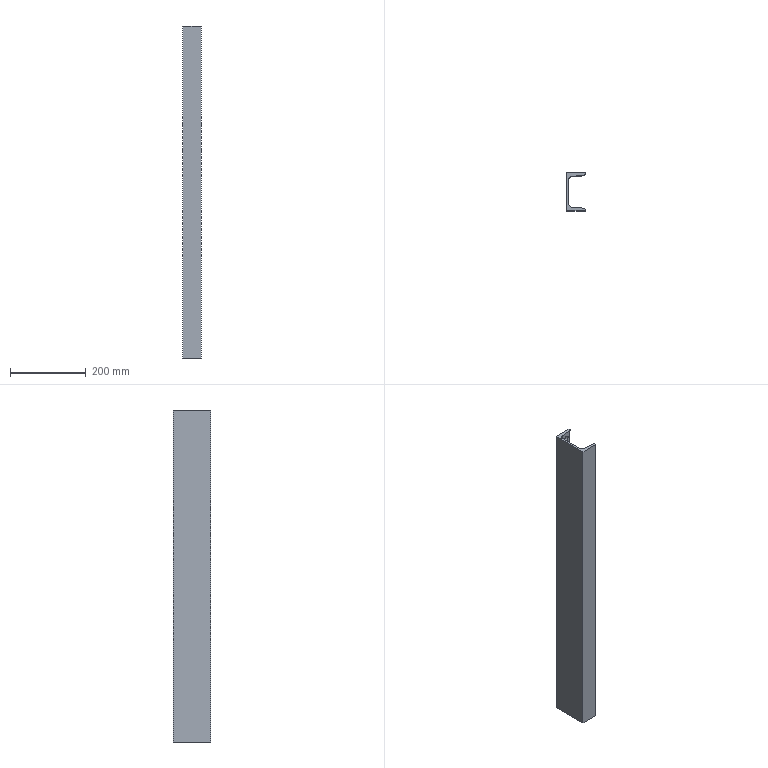Part | NX | features BREP 1, DATUM_CSYS 1, SKETCH 1 | 1 solid | 24 faces | box 48 x 100 x 876 mm | volume 1087998 mm3 | cylinder 14 | plane 10 | commonest cylinder face diameters 14 x10 8.4 x2 17 x2
STEP:
#1=CARTESIAN_POINT('',(30.,92.079,203.));
#2=VERTEX_POINT('',#1);
#3=CARTESIAN_POINT('',(30.,92.079,217.));
#4=VERTEX_POINT('',#3);
#5=CARTESIAN_POINT('',(30.,92.079,203.));
#6=CARTESIAN_POINT('',(16.,90.926,203.));
#7=CARTESIAN_POINT('',(16.,90.926,217.));
#8=CARTESIAN_POINT('',(30.,92.079,217.));
#9=(BOUNDED_CURVE()B_SPLINE_CURVE(3,(#5,#6,#7,#8),.UNSPECIFIED.,.F.,.F.)B_SPLINE_CURVE_WITH_KNOTS((4,4),(0.,1.),.PIECEWISE_BEZIER_KNOTS.)CURVE()GEOMETRIC_REPRESENTATION_ITEM()RATIONAL_B_SPLINE_CURVE((1.,0.3333,0.3333,1.))REPRESENTATION_ITEM(''));
#10=EDGE_CURVE('',#2,#4,#9,.T.);
#11=ORIENTED_EDGE('',*,*,#10,.F.);
#12=CARTESIAN_POINT('',(30.,100.,203.));
#13=VERTEX_POINT('',#12);
#14=CARTESIAN_POINT('',(30.,70.,203.));
#15=DIRECTION('',(0.,1.,0.));
#16=VECTOR('',#15,1000.);
#17=LINE('',#14,#16);
#18=EDGE_CURVE('',#2,#13,#17,.T.);
#19=ORIENTED_EDGE('',*,*,#18,.T.);
#20=CARTESIAN_POINT('',(30.,100.,217.));
#21=VERTEX_POINT('',#20);
#22=CARTESIAN_POINT('',(30.,100.,210.));
#23=DIRECTION('',(0.,1.,0.));
#24=DIRECTION('',(0.,0.,-1.));
#25=AXIS2_PLACEMENT_3D('',#22,#23,#24);
#26=CIRCLE('',#25,7.);
#27=EDGE_CURVE('',#13,#21,#26,.T.);
#28=ORIENTED_EDGE('',*,*,#27,.T.);
#29=CARTESIAN_POINT('',(30.,70.,217.));
#30=DIRECTION('',(0.,1.,0.));
#31=VECTOR('',#30,1000.);
#32=LINE('',#29,#31);
#33=EDGE_CURVE('',#4,#21,#32,.T.);
#34=ORIENTED_EDGE('',*,*,#33,.F.);
#35=EDGE_LOOP('',(#11,#19,#28,#34));
#36=FACE_BOUND('',#35,.T.);
#37=CARTESIAN_POINT('',(30.,70.,210.));
#38=DIRECTION('',(0.,1.,0.));
#39=DIRECTION('',(0.,0.,-1.));
#40=AXIS2_PLACEMENT_3D('',#37,#38,#39);
#41=CYLINDRICAL_SURFACE('',#40,7.);
#42=ADVANCED_FACE('',(#36),#41,.F.);
#43=CARTESIAN_POINT('',(30.,92.079,413.));
#44=VERTEX_POINT('',#43);
#45=CARTESIAN_POINT('',(30.,92.079,427.));
#46=VERTEX_POINT('',#45);
#47=CARTESIAN_POINT('',(30.,92.079,413.));
#48=CARTESIAN_POINT('',(16.,90.926,413.));
#49=CARTESIAN_POINT('',(16.,90.926,427.));
#50=CARTESIAN_POINT('',(30.,92.079,427.));
#51=(BOUNDED_CURVE()B_SPLINE_CURVE(3,(#47,#48,#49,#50),.UNSPECIFIED.,.F.,.F.)B_SPLINE_CURVE_WITH_KNOTS((4,4),(0.,1.),.PIECEWISE_BEZIER_KNOTS.)CURVE()GEOMETRIC_REPRESENTATION_ITEM()RATIONAL_B_SPLINE_CURVE((1.,0.3333,0.3333,1.))REPRESENTATION_ITEM(''));
#52=EDGE_CURVE('',#44,#46,#51,.T.);
#53=ORIENTED_EDGE('',*,*,#52,.F.);
#54=CARTESIAN_POINT('',(30.,100.,413.));
#55=VERTEX_POINT('',#54);
#56=CARTESIAN_POINT('',(30.,70.,413.));
#57=DIRECTION('',(0.,1.,0.));
#58=VECTOR('',#57,1000.);
#59=LINE('',#56,#58);
#60=EDGE_CURVE('',#44,#55,#59,.T.);
#61=ORIENTED_EDGE('',*,*,#60,.T.);
#62=CARTESIAN_POINT('',(30.,100.,427.));
#63=VERTEX_POINT('',#62);
#64=CARTESIAN_POINT('',(30.,100.,420.));
#65=DIRECTION('',(0.,1.,0.));
#66=DIRECTION('',(0.,0.,-1.));
#67=AXIS2_PLACEMENT_3D('',#64,#65,#66);
#68=CIRCLE('',#67,7.);
#69=EDGE_CURVE('',#55,#63,#68,.T.);
#70=ORIENTED_EDGE('',*,*,#69,.T.);
#71=CARTESIAN_POINT('',(30.,70.,427.));
#72=DIRECTION('',(0.,1.,0.));
#73=VECTOR('',#72,1000.);
#74=LINE('',#71,#73);
#75=EDGE_CURVE('',#46,#63,#74,.T.);
#76=ORIENTED_EDGE('',*,*,#75,.F.);
#77=EDGE_LOOP('',(#53,#61,#70,#76));
#78=FACE_BOUND('',#77,.T.);
#79=CARTESIAN_POINT('',(30.,70.,420.));
#80=DIRECTION('',(0.,1.,0.));
#81=DIRECTION('',(0.,0.,-1.));
#82=AXIS2_PLACEMENT_3D('',#79,#80,#81);
#83=CYLINDRICAL_SURFACE('',#82,7.);
#84=ADVANCED_FACE('',(#78),#83,.F.);
#85=CARTESIAN_POINT('',(30.,92.079,-427.));
#86=VERTEX_POINT('',#85);
#87=CARTESIAN_POINT('',(30.,92.079,-413.));
#88=VERTEX_POINT('',#87);
#89=CARTESIAN_POINT('',(30.,92.079,-427.));
#90=CARTESIAN_POINT('',(16.,90.926,-427.));
#91=CARTESIAN_POINT('',(16.,90.926,-413.));
#92=CARTESIAN_POINT('',(30.,92.079,-413.));
#93=(BOUNDED_CURVE()B_SPLINE_CURVE(3,(#89,#90,#91,#92),.UNSPECIFIED.,.F.,.F.)B_SPLINE_CURVE_WITH_KNOTS((4,4),(0.,1.),.PIECEWISE_BEZIER_KNOTS.)CURVE()GEOMETRIC_REPRESENTATION_ITEM()RATIONAL_B_SPLINE_CURVE((1.,0.3333,0.3333,1.))REPRESENTATION_ITEM(''));
#94=EDGE_CURVE('',#86,#88,#93,.T.);
#95=ORIENTED_EDGE('',*,*,#94,.F.);
#96=CARTESIAN_POINT('',(30.,100.,-427.));
#97=VERTEX_POINT('',#96);
#98=CARTESIAN_POINT('',(30.,70.,-427.));
#99=DIRECTION('',(0.,1.,0.));
#100=VECTOR('',#99,1000.);
#101=LINE('',#98,#100);
#102=EDGE_CURVE('',#86,#97,#101,.T.);
#103=ORIENTED_EDGE('',*,*,#102,.T.);
#104=CARTESIAN_POINT('',(30.,100.,-413.));
#105=VERTEX_POINT('',#104);
#106=CARTESIAN_POINT('',(30.,100.,-420.));
#107=DIRECTION('',(0.,1.,0.));
#108=DIRECTION('',(0.,0.,1.));
#109=AXIS2_PLACEMENT_3D('',#106,#107,#108);
#110=CIRCLE('',#109,7.);
#111=EDGE_CURVE('',#97,#105,#110,.T.);
#112=ORIENTED_EDGE('',*,*,#111,.T.);
#113=CARTESIAN_POINT('',(30.,70.,-413.));
#114=DIRECTION('',(0.,1.,0.));
#115=VECTOR('',#114,1000.);
#116=LINE('',#113,#115);
#117=EDGE_CURVE('',#88,#105,#116,.T.);
#118=ORIENTED_EDGE('',*,*,#117,.F.);
#119=EDGE_LOOP('',(#95,#103,#112,#118));
#120=FACE_BOUND('',#119,.T.);
#121=CARTESIAN_POINT('',(30.,70.,-420.));
#122=DIRECTION('',(0.,1.,0.));
#123=DIRECTION('',(0.,0.,-1.));
#124=AXIS2_PLACEMENT_3D('',#121,#122,#123);
#125=CYLINDRICAL_SURFACE('',#124,7.);
#126=ADVANCED_FACE('',(#120),#125,.F.);
#127=CARTESIAN_POINT('',(30.,92.079,-217.));
#128=VERTEX_POINT('',#127);
#129=CARTESIAN_POINT('',(30.,92.079,-203.));
#130=VERTEX_POINT('',#129);
#131=CARTESIAN_POINT('',(30.,92.079,-217.));
#132=CARTESIAN_POINT('',(16.,90.926,-217.));
#133=CARTESIAN_POINT('',(16.,90.926,-203.));
#134=CARTESIAN_POINT('',(30.,92.079,-203.));
#135=(BOUNDED_CURVE()B_SPLINE_CURVE(3,(#131,#132,#133,#134),.UNSPECIFIED.,.F.,.F.)B_SPLINE_CURVE_WITH_KNOTS((4,4),(0.,1.),.PIECEWISE_BEZIER_KNOTS.)CURVE()GEOMETRIC_REPRESENTATION_ITEM()RATIONAL_B_SPLINE_CURVE((1.,0.3333,0.3333,1.))REPRESENTATION_ITEM(''));
#136=EDGE_CURVE('',#128,#130,#135,.T.);
#137=ORIENTED_EDGE('',*,*,#136,.F.);
#138=CARTESIAN_POINT('',(30.,100.,-217.));
#139=VERTEX_POINT('',#138);
#140=CARTESIAN_POINT('',(30.,70.,-217.));
#141=DIRECTION('',(0.,1.,0.));
#142=VECTOR('',#141,1000.);
#143=LINE('',#140,#142);
#144=EDGE_CURVE('',#128,#139,#143,.T.);
#145=ORIENTED_EDGE('',*,*,#144,.T.);
#146=CARTESIAN_POINT('',(30.,100.,-203.));
#147=VERTEX_POINT('',#146);
#148=CARTESIAN_POINT('',(30.,100.,-210.));
#149=DIRECTION('',(0.,1.,0.));
#150=DIRECTION('',(0.,0.,1.));
#151=AXIS2_PLACEMENT_3D('',#148,#149,#150);
#152=CIRCLE('',#151,7.);
#153=EDGE_CURVE('',#139,#147,#152,.T.);
#154=ORIENTED_EDGE('',*,*,#153,.T.);
#155=CARTESIAN_POINT('',(30.,70.,-203.));
#156=DIRECTION('',(0.,1.,0.));
#157=VECTOR('',#156,1000.);
#158=LINE('',#155,#157);
#159=EDGE_CURVE('',#130,#147,#158,.T.);
#160=ORIENTED_EDGE('',*,*,#159,.F.);
#161=EDGE_LOOP('',(#137,#145,#154,#160));
#162=FACE_BOUND('',#161,.T.);
#163=CARTESIAN_POINT('',(30.,70.,-210.));
#164=DIRECTION('',(0.,1.,0.));
#165=DIRECTION('',(0.,0.,-1.));
#166=AXIS2_PLACEMENT_3D('',#163,#164,#165);
#167=CYLINDRICAL_SURFACE('',#166,7.);
#168=ADVANCED_FACE('',(#162),#167,.F.);
#169=CARTESIAN_POINT('',(30.,92.079,-7.));
#170=VERTEX_POINT('',#169);
#171=CARTESIAN_POINT('',(30.,92.079,7.));
#172=VERTEX_POINT('',#171);
#173=CARTESIAN_POINT('',(30.,92.079,-7.));
#174=CARTESIAN_POINT('',(16.,90.926,-7.));
#175=CARTESIAN_POINT('',(16.,90.926,7.));
#176=CARTESIAN_POINT('',(30.,92.079,7.));
#177=(BOUNDED_CURVE()B_SPLINE_CURVE(3,(#173,#174,#175,#176),.UNSPECIFIED.,.F.,.F.)B_SPLINE_CURVE_WITH_KNOTS((4,4),(0.,1.),.PIECEWISE_BEZIER_KNOTS.)CURVE()GEOMETRIC_REPRESENTATION_ITEM()RATIONAL_B_SPLINE_CURVE((1.,0.3333,0.3333,1.))REPRESENTATION_ITEM(''));
#178=EDGE_CURVE('',#170,#172,#177,.T.);
#179=ORIENTED_EDGE('',*,*,#178,.F.);
#180=CARTESIAN_POINT('',(30.,100.,-7.));
#181=VERTEX_POINT('',#180);
#182=CARTESIAN_POINT('',(30.,70.,-7.));
#183=DIRECTION('',(0.,1.,0.));
#184=VECTOR('',#183,1000.);
#185=LINE('',#182,#184);
#186=EDGE_CURVE('',#170,#181,#185,.T.);
#187=ORIENTED_EDGE('',*,*,#186,.T.);
#188=CARTESIAN_POINT('',(30.,100.,7.));
#189=VERTEX_POINT('',#188);
#190=CARTESIAN_POINT('',(30.,100.,0.));
#191=DIRECTION('',(0.,1.,0.));
#192=DIRECTION('',(0.,0.,1.));
#193=AXIS2_PLACEMENT_3D('',#190,#191,#192);
#194=CIRCLE('',#193,7.);
#195=EDGE_CURVE('',#181,#189,#194,.T.);
#196=ORIENTED_EDGE('',*,*,#195,.T.);
#197=CARTESIAN_POINT('',(30.,70.,7.));
#198=DIRECTION('',(0.,1.,0.));
#199=VECTOR('',#198,1000.);
#200=LINE('',#197,#199);
#201=EDGE_CURVE('',#172,#189,#200,.T.);
#202=ORIENTED_EDGE('',*,*,#201,.F.);
#203=EDGE_LOOP('',(#179,#187,#196,#202));
#204=FACE_BOUND('',#203,.T.);
#205=CARTESIAN_POINT('',(30.,70.,0.));
#206=DIRECTION('',(0.,1.,0.));
#207=DIRECTION('',(0.,0.,-1.));
#208=AXIS2_PLACEMENT_3D('',#205,#206,#207);
#209=CYLINDRICAL_SURFACE('',#208,7.);
#210=ADVANCED_FACE('',(#204),#209,.F.);
#211=CARTESIAN_POINT('',(0.,0.,-438.));
#212=VERTEX_POINT('',#211);
#213=CARTESIAN_POINT('',(48.,0.,-438.));
#214=VERTEX_POINT('',#213);
#215=CARTESIAN_POINT('',(0.,0.,-438.));
#216=DIRECTION('',(1.,0.,0.));
#217=VECTOR('',#216,1000.);
#218=LINE('',#215,#217);
#219=EDGE_CURVE('',#212,#214,#218,.T.);
#220=ORIENTED_EDGE('',*,*,#219,.T.);
#221=CARTESIAN_POINT('',(48.,0.,438.));
#222=VERTEX_POINT('',#221);
#223=CARTESIAN_POINT('',(48.,0.,438.));
#224=DIRECTION('',(0.,0.,-1.));
#225=VECTOR('',#224,1000.);
#226=LINE('',#223,#225);
#227=EDGE_CURVE('',#222,#214,#226,.T.);
#228=ORIENTED_EDGE('',*,*,#227,.F.);
#229=CARTESIAN_POINT('',(0.,0.,438.));
#230=VERTEX_POINT('',#229);
#231=CARTESIAN_POINT('',(0.,0.,438.));
#232=DIRECTION('',(1.,0.,0.));
#233=VECTOR('',#232,1000.);
#234=LINE('',#231,#233);
#235=EDGE_CURVE('',#230,#222,#234,.T.);
#236=ORIENTED_EDGE('',*,*,#235,.F.);
#237=CARTESIAN_POINT('',(0.,0.,438.));
#238=DIRECTION('',(0.,0.,-1.));
#239=VECTOR('',#238,1000.);
#240=LINE('',#237,#239);
#241=EDGE_CURVE('',#230,#212,#240,.T.);
#242=ORIENTED_EDGE('',*,*,#241,.T.);
#243=EDGE_LOOP('',(#220,#228,#236,#242));
#244=FACE_BOUND('',#243,.T.);
#245=CARTESIAN_POINT('',(0.,0.,438.));
#246=DIRECTION('',(0.,1.,0.));
#247=DIRECTION('',(0.,0.,-1.));
#248=AXIS2_PLACEMENT_3D('',#245,#246,#247);
#249=PLANE('',#248);
#250=ADVANCED_FACE('',(#244),#249,.F.);
#251=CARTESIAN_POINT('',(48.,2.585,-438.));
#252=VERTEX_POINT('',#251);
#253=CARTESIAN_POINT('',(48.,0.,-438.));
#254=DIRECTION('',(0.,1.,0.));
#255=VECTOR('',#254,1000.);
#256=LINE('',#253,#255);
#257=EDGE_CURVE('',#214,#252,#256,.T.);
#258=ORIENTED_EDGE('',*,*,#257,.T.);
#259=CARTESIAN_POINT('',(48.,2.585,438.));
#260=VERTEX_POINT('',#259);
#261=CARTESIAN_POINT('',(48.,2.585,438.));
#262=DIRECTION('',(0.,0.,-1.));
#263=VECTOR('',#262,1000.);
#264=LINE('',#261,#263);
#265=EDGE_CURVE('',#260,#252,#264,.T.);
#266=ORIENTED_EDGE('',*,*,#265,.F.);
#267=CARTESIAN_POINT('',(48.,0.,438.));
#268=DIRECTION('',(0.,1.,0.));
#269=VECTOR('',#268,1000.);
#270=LINE('',#267,#269);
#271=EDGE_CURVE('',#222,#260,#270,.T.);
#272=ORIENTED_EDGE('',*,*,#271,.F.);
#273=ORIENTED_EDGE('',*,*,#227,.T.);
#274=EDGE_LOOP('',(#258,#266,#272,#273));
#275=FACE_BOUND('',#274,.T.);
#276=CARTESIAN_POINT('',(48.,0.,438.));
#277=DIRECTION('',(-1.,0.,0.));
#278=DIRECTION('',(0.,0.,-1.));
#279=AXIS2_PLACEMENT_3D('',#276,#277,#278);
#280=PLANE('',#279);
#281=ADVANCED_FACE('',(#275),#280,.F.);
#282=CARTESIAN_POINT('',(43.8,6.785,-438.));
#283=VERTEX_POINT('',#282);
#284=CARTESIAN_POINT('',(43.8,2.585,-438.));
#285=DIRECTION('',(0.,0.,1.));
#286=DIRECTION('',(1.,0.,0.));
#287=AXIS2_PLACEMENT_3D('',#284,#285,#286);
#288=CIRCLE('',#287,4.2);
#289=EDGE_CURVE('',#252,#283,#288,.T.);
#290=ORIENTED_EDGE('',*,*,#289,.T.);
#291=CARTESIAN_POINT('',(43.8,6.785,438.));
#292=VERTEX_POINT('',#291);
#293=CARTESIAN_POINT('',(43.8,6.785,438.));
#294=DIRECTION('',(0.,0.,-1.));
#295=VECTOR('',#294,1000.);
#296=LINE('',#293,#295);
#297=EDGE_CURVE('',#292,#283,#296,.T.);
#298=ORIENTED_EDGE('',*,*,#297,.F.);
#299=CARTESIAN_POINT('',(43.8,2.585,438.));
#300=DIRECTION('',(0.,0.,1.));
#301=DIRECTION('',(1.,0.,0.));
#302=AXIS2_PLACEMENT_3D('',#299,#300,#301);
#303=CIRCLE('',#302,4.2);
#304=EDGE_CURVE('',#260,#292,#303,.T.);
#305=ORIENTED_EDGE('',*,*,#304,.F.);
#306=ORIENTED_EDGE('',*,*,#265,.T.);
#307=EDGE_LOOP('',(#290,#298,#305,#306));
#308=FACE_BOUND('',#307,.T.);
#309=CARTESIAN_POINT('',(43.8,2.585,438.));
#310=DIRECTION('',(0.,0.,-1.));
#311=DIRECTION('',(1.,0.,0.));
#312=AXIS2_PLACEMENT_3D('',#309,#310,#311);
#313=CYLINDRICAL_SURFACE('',#312,4.2);
#314=ADVANCED_FACE('',(#308),#313,.T.);
#315=CARTESIAN_POINT('',(13.8,9.255,-438.));
#316=VERTEX_POINT('',#315);
#317=CARTESIAN_POINT('',(43.8,6.785,-438.));
#318=DIRECTION('',(-0.9966,0.08206,0.));
#319=VECTOR('',#318,1000.);
#320=LINE('',#317,#319);
#321=EDGE_CURVE('',#283,#316,#320,.T.);
#322=ORIENTED_EDGE('',*,*,#321,.T.);
#323=CARTESIAN_POINT('',(13.8,9.255,438.));
#324=VERTEX_POINT('',#323);
#325=CARTESIAN_POINT('',(13.8,9.255,438.));
#326=DIRECTION('',(0.,0.,-1.));
#327=VECTOR('',#326,1000.);
#328=LINE('',#325,#327);
#329=EDGE_CURVE('',#324,#316,#328,.T.);
#330=ORIENTED_EDGE('',*,*,#329,.F.);
#331=CARTESIAN_POINT('',(43.8,6.785,438.));
#332=DIRECTION('',(-0.9966,0.08206,0.));
#333=VECTOR('',#332,1000.);
#334=LINE('',#331,#333);
#335=EDGE_CURVE('',#292,#324,#334,.T.);
#336=ORIENTED_EDGE('',*,*,#335,.F.);
#337=ORIENTED_EDGE('',*,*,#297,.T.);
#338=EDGE_LOOP('',(#322,#330,#336,#337));
#339=FACE_BOUND('',#338,.T.);
#340=CARTESIAN_POINT('',(43.8,6.785,438.));
#341=DIRECTION('',(-0.08206,-0.9966,0.));
#342=DIRECTION('',(-0.9966,0.08206,0.));
#343=AXIS2_PLACEMENT_3D('',#340,#341,#342);
#344=PLANE('',#343);
#345=ADVANCED_FACE('',(#339),#344,.F.);
#346=CARTESIAN_POINT('',(5.3,17.755,-438.));
#347=VERTEX_POINT('',#346);
#348=CARTESIAN_POINT('',(13.8,17.755,-438.));
#349=DIRECTION('',(0.,0.,-1.));
#350=DIRECTION('',(1.,0.,0.));
#351=AXIS2_PLACEMENT_3D('',#348,#349,#350);
#352=CIRCLE('',#351,8.5);
#353=EDGE_CURVE('',#316,#347,#352,.T.);
#354=ORIENTED_EDGE('',*,*,#353,.T.);
#355=CARTESIAN_POINT('',(5.3,17.755,438.));
#356=VERTEX_POINT('',#355);
#357=CARTESIAN_POINT('',(5.3,17.755,438.));
#358=DIRECTION('',(0.,0.,-1.));
#359=VECTOR('',#358,1000.);
#360=LINE('',#357,#359);
#361=EDGE_CURVE('',#356,#347,#360,.T.);
#362=ORIENTED_EDGE('',*,*,#361,.F.);
#363=CARTESIAN_POINT('',(13.8,17.755,438.));
#364=DIRECTION('',(0.,0.,-1.));
#365=DIRECTION('',(1.,0.,0.));
#366=AXIS2_PLACEMENT_3D('',#363,#364,#365);
#367=CIRCLE('',#366,8.5);
#368=EDGE_CURVE('',#324,#356,#367,.T.);
#369=ORIENTED_EDGE('',*,*,#368,.F.);
#370=ORIENTED_EDGE('',*,*,#329,.T.);
#371=EDGE_LOOP('',(#354,#362,#369,#370));
#372=FACE_BOUND('',#371,.T.);
#373=CARTESIAN_POINT('',(13.8,17.755,438.));
#374=DIRECTION('',(0.,0.,-1.));
#375=DIRECTION('',(1.,0.,0.));
#376=AXIS2_PLACEMENT_3D('',#373,#374,#375);
#377=CYLINDRICAL_SURFACE('',#376,8.5);
#378=ADVANCED_FACE('',(#372),#377,.F.);
#379=CARTESIAN_POINT('',(5.3,82.245,-438.));
#380=VERTEX_POINT('',#379);
#381=CARTESIAN_POINT('',(5.3,17.755,-438.));
#382=DIRECTION('',(0.,1.,0.));
#383=VECTOR('',#382,1000.);
#384=LINE('',#381,#383);
#385=EDGE_CURVE('',#347,#380,#384,.T.);
#386=ORIENTED_EDGE('',*,*,#385,.T.);
#387=CARTESIAN_POINT('',(5.3,82.245,438.));
#388=VERTEX_POINT('',#387);
#389=CARTESIAN_POINT('',(5.3,82.245,438.));
#390=DIRECTION('',(0.,0.,-1.));
#391=VECTOR('',#390,1000.);
#392=LINE('',#389,#391);
#393=EDGE_CURVE('',#388,#380,#392,.T.);
#394=ORIENTED_EDGE('',*,*,#393,.F.);
#395=CARTESIAN_POINT('',(5.3,17.755,438.));
#396=DIRECTION('',(0.,1.,0.));
#397=VECTOR('',#396,1000.);
#398=LINE('',#395,#397);
#399=EDGE_CURVE('',#356,#388,#398,.T.);
#400=ORIENTED_EDGE('',*,*,#399,.F.);
#401=ORIENTED_EDGE('',*,*,#361,.T.);
#402=EDGE_LOOP('',(#386,#394,#400,#401));
#403=FACE_BOUND('',#402,.T.);
#404=CARTESIAN_POINT('',(5.3,17.755,438.));
#405=DIRECTION('',(-1.,0.,0.));
#406=DIRECTION('',(0.,0.,-1.));
#407=AXIS2_PLACEMENT_3D('',#404,#405,#406);
#408=PLANE('',#407);
#409=ADVANCED_FACE('',(#403),#408,.F.);
#410=CARTESIAN_POINT('',(13.8,90.745,-438.));
#411=VERTEX_POINT('',#410);
#412=CARTESIAN_POINT('',(13.8,82.245,-438.));
#413=DIRECTION('',(0.,0.,-1.));
#414=DIRECTION('',(-1.,0.,0.));
#415=AXIS2_PLACEMENT_3D('',#412,#413,#414);
#416=CIRCLE('',#415,8.5);
#417=EDGE_CURVE('',#380,#411,#416,.T.);
#418=ORIENTED_EDGE('',*,*,#417,.T.);
#419=CARTESIAN_POINT('',(13.8,90.745,438.));
#420=VERTEX_POINT('',#419);
#421=CARTESIAN_POINT('',(13.8,90.745,438.));
#422=DIRECTION('',(0.,0.,-1.));
#423=VECTOR('',#422,1000.);
#424=LINE('',#421,#423);
#425=EDGE_CURVE('',#420,#411,#424,.T.);
#426=ORIENTED_EDGE('',*,*,#425,.F.);
#427=CARTESIAN_POINT('',(13.8,82.245,438.));
#428=DIRECTION('',(0.,0.,-1.));
#429=DIRECTION('',(-1.,0.,0.));
#430=AXIS2_PLACEMENT_3D('',#427,#428,#429);
#431=CIRCLE('',#430,8.5);
#432=EDGE_CURVE('',#388,#420,#431,.T.);
#433=ORIENTED_EDGE('',*,*,#432,.F.);
#434=ORIENTED_EDGE('',*,*,#393,.T.);
#435=EDGE_LOOP('',(#418,#426,#433,#434));
#436=FACE_BOUND('',#435,.T.);
#437=CARTESIAN_POINT('',(13.8,82.245,438.));
#438=DIRECTION('',(0.,0.,-1.));
#439=DIRECTION('',(1.,0.,0.));
#440=AXIS2_PLACEMENT_3D('',#437,#438,#439);
#441=CYLINDRICAL_SURFACE('',#440,8.5);
#442=ADVANCED_FACE('',(#436),#441,.F.);
#443=CARTESIAN_POINT('',(30.,92.079,217.));
#444=CARTESIAN_POINT('',(44.,93.231,217.));
#445=CARTESIAN_POINT('',(44.,93.231,203.));
#446=CARTESIAN_POINT('',(30.,92.079,203.));
#447=(BOUNDED_CURVE()B_SPLINE_CURVE(3,(#443,#444,#445,#446),.UNSPECIFIED.,.F.,.F.)B_SPLINE_CURVE_WITH_KNOTS((4,4),(0.,1.),.PIECEWISE_BEZIER_KNOTS.)CURVE()GEOMETRIC_REPRESENTATION_ITEM()RATIONAL_B_SPLINE_CURVE((1.,0.3333,0.3333,1.))REPRESENTATION_ITEM(''));
#448=EDGE_CURVE('',#4,#2,#447,.T.);
#449=ORIENTED_EDGE('',*,*,#448,.T.);
#450=ORIENTED_EDGE('',*,*,#10,.T.);
#451=EDGE_LOOP('',(#449,#450));
#452=FACE_BOUND('',#451,.T.);
#453=CARTESIAN_POINT('',(30.,92.079,427.));
#454=CARTESIAN_POINT('',(44.,93.231,427.));
#455=CARTESIAN_POINT('',(44.,93.231,413.));
#456=CARTESIAN_POINT('',(30.,92.079,413.));
#457=(BOUNDED_CURVE()B_SPLINE_CURVE(3,(#453,#454,#455,#456),.UNSPECIFIED.,.F.,.F.)B_SPLINE_CURVE_WITH_KNOTS((4,4),(0.,1.),.PIECEWISE_BEZIER_KNOTS.)CURVE()GEOMETRIC_REPRESENTATION_ITEM()RATIONAL_B_SPLINE_CURVE((1.,0.3333,0.3333,1.))REPRESENTATION_ITEM(''));
#458=EDGE_CURVE('',#46,#44,#457,.T.);
#459=ORIENTED_EDGE('',*,*,#458,.T.);
#460=ORIENTED_EDGE('',*,*,#52,.T.);
#461=EDGE_LOOP('',(#459,#460));
#462=FACE_BOUND('',#461,.T.);
#463=CARTESIAN_POINT('',(30.,92.079,-413.));
#464=CARTESIAN_POINT('',(44.,93.231,-413.));
#465=CARTESIAN_POINT('',(44.,93.231,-427.));
#466=CARTESIAN_POINT('',(30.,92.079,-427.));
#467=(BOUNDED_CURVE()B_SPLINE_CURVE(3,(#463,#464,#465,#466),.UNSPECIFIED.,.F.,.F.)B_SPLINE_CURVE_WITH_KNOTS((4,4),(0.,1.),.PIECEWISE_BEZIER_KNOTS.)CURVE()GEOMETRIC_REPRESENTATION_ITEM()RATIONAL_B_SPLINE_CURVE((1.,0.3333,0.3333,1.))REPRESENTATION_ITEM(''));
#468=EDGE_CURVE('',#88,#86,#467,.T.);
#469=ORIENTED_EDGE('',*,*,#468,.T.);
#470=ORIENTED_EDGE('',*,*,#94,.T.);
#471=EDGE_LOOP('',(#469,#470));
#472=FACE_BOUND('',#471,.T.);
#473=CARTESIAN_POINT('',(30.,92.079,-203.));
#474=CARTESIAN_POINT('',(44.,93.231,-203.));
#475=CARTESIAN_POINT('',(44.,93.231,-217.));
#476=CARTESIAN_POINT('',(30.,92.079,-217.));
#477=(BOUNDED_CURVE()B_SPLINE_CURVE(3,(#473,#474,#475,#476),.UNSPECIFIED.,.F.,.F.)B_SPLINE_CURVE_WITH_KNOTS((4,4),(0.,1.),.PIECEWISE_BEZIER_KNOTS.)CURVE()GEOMETRIC_REPRESENTATION_ITEM()RATIONAL_B_SPLINE_CURVE((1.,0.3333,0.3333,1.))REPRESENTATION_ITEM(''));
#478=EDGE_CURVE('',#130,#128,#477,.T.);
#479=ORIENTED_EDGE('',*,*,#478,.T.);
#480=ORIENTED_EDGE('',*,*,#136,.T.);
#481=EDGE_LOOP('',(#479,#480));
#482=FACE_BOUND('',#481,.T.);
#483=CARTESIAN_POINT('',(30.,92.079,7.));
#484=CARTESIAN_POINT('',(44.,93.231,7.));
#485=CARTESIAN_POINT('',(44.,93.231,-7.));
#486=CARTESIAN_POINT('',(30.,92.079,-7.));
#487=(BOUNDED_CURVE()B_SPLINE_CURVE(3,(#483,#484,#485,#486),.UNSPECIFIED.,.F.,.F.)B_SPLINE_CURVE_WITH_KNOTS((4,4),(0.,1.),.PIECEWISE_BEZIER_KNOTS.)CURVE()GEOMETRIC_REPRESENTATION_ITEM()RATIONAL_B_SPLINE_CURVE((1.,0.3333,0.3333,1.))REPRESENTATION_ITEM(''));
#488=EDGE_CURVE('',#172,#170,#487,.T.);
#489=ORIENTED_EDGE('',*,*,#488,.T.);
#490=ORIENTED_EDGE('',*,*,#178,.T.);
#491=EDGE_LOOP('',(#489,#490));
#492=FACE_BOUND('',#491,.T.);
#493=CARTESIAN_POINT('',(43.8,93.215,-438.));
#494=VERTEX_POINT('',#493);
#495=CARTESIAN_POINT('',(43.8,93.215,-438.));
#496=DIRECTION('',(0.9966,0.08206,0.));
#497=VECTOR('',#496,1000.);
#498=LINE('',#495,#497);
#499=EDGE_CURVE('',#411,#494,#498,.T.);
#500=ORIENTED_EDGE('',*,*,#499,.T.);
#501=CARTESIAN_POINT('',(43.8,93.215,438.));
#502=VERTEX_POINT('',#501);
#503=CARTESIAN_POINT('',(43.8,93.215,438.));
#504=DIRECTION('',(0.,0.,-1.));
#505=VECTOR('',#504,1000.);
#506=LINE('',#503,#505);
#507=EDGE_CURVE('',#502,#494,#506,.T.);
#508=ORIENTED_EDGE('',*,*,#507,.F.);
#509=CARTESIAN_POINT('',(43.8,93.215,438.));
#510=DIRECTION('',(0.9966,0.08206,0.));
#511=VECTOR('',#510,1000.);
#512=LINE('',#509,#511);
#513=EDGE_CURVE('',#420,#502,#512,.T.);
#514=ORIENTED_EDGE('',*,*,#513,.F.);
#515=ORIENTED_EDGE('',*,*,#425,.T.);
#516=EDGE_LOOP('',(#500,#508,#514,#515));
#517=FACE_BOUND('',#516,.T.);
#518=CARTESIAN_POINT('',(43.8,93.215,438.));
#519=DIRECTION('',(-0.08206,0.9966,0.));
#520=DIRECTION('',(0.9966,0.08206,0.));
#521=AXIS2_PLACEMENT_3D('',#518,#519,#520);
#522=PLANE('',#521);
#523=ADVANCED_FACE('',(#452,#462,#472,#482,#492,#517),#522,.F.);
#524=CARTESIAN_POINT('',(48.,97.415,-438.));
#525=VERTEX_POINT('',#524);
#526=CARTESIAN_POINT('',(43.8,97.415,-438.));
#527=DIRECTION('',(0.,0.,1.));
#528=DIRECTION('',(-1.,0.,0.));
#529=AXIS2_PLACEMENT_3D('',#526,#527,#528);
#530=CIRCLE('',#529,4.2);
#531=EDGE_CURVE('',#494,#525,#530,.T.);
#532=ORIENTED_EDGE('',*,*,#531,.T.);
#533=CARTESIAN_POINT('',(48.,97.415,438.));
#534=VERTEX_POINT('',#533);
#535=CARTESIAN_POINT('',(48.,97.415,438.));
#536=DIRECTION('',(0.,0.,-1.));
#537=VECTOR('',#536,1000.);
#538=LINE('',#535,#537);
#539=EDGE_CURVE('',#534,#525,#538,.T.);
#540=ORIENTED_EDGE('',*,*,#539,.F.);
#541=CARTESIAN_POINT('',(43.8,97.415,438.));
#542=DIRECTION('',(0.,0.,1.));
#543=DIRECTION('',(-1.,0.,0.));
#544=AXIS2_PLACEMENT_3D('',#541,#542,#543);
#545=CIRCLE('',#544,4.2);
#546=EDGE_CURVE('',#502,#534,#545,.T.);
#547=ORIENTED_EDGE('',*,*,#546,.F.);
#548=ORIENTED_EDGE('',*,*,#507,.T.);
#549=EDGE_LOOP('',(#532,#540,#547,#548));
#550=FACE_BOUND('',#549,.T.);
#551=CARTESIAN_POINT('',(43.8,97.415,438.));
#552=DIRECTION('',(0.,0.,-1.));
#553=DIRECTION('',(1.,0.,0.));
#554=AXIS2_PLACEMENT_3D('',#551,#552,#553);
#555=CYLINDRICAL_SURFACE('',#554,4.2);
#556=ADVANCED_FACE('',(#550),#555,.T.);
#557=CARTESIAN_POINT('',(48.,100.,-438.));
#558=VERTEX_POINT('',#557);
#559=CARTESIAN_POINT('',(48.,100.,-438.));
#560=DIRECTION('',(0.,1.,0.));
#561=VECTOR('',#560,1000.);
#562=LINE('',#559,#561);
#563=EDGE_CURVE('',#525,#558,#562,.T.);
#564=ORIENTED_EDGE('',*,*,#563,.T.);
#565=CARTESIAN_POINT('',(48.,100.,438.));
#566=VERTEX_POINT('',#565);
#567=CARTESIAN_POINT('',(48.,100.,438.));
#568=DIRECTION('',(0.,0.,-1.));
#569=VECTOR('',#568,1000.);
#570=LINE('',#567,#569);
#571=EDGE_CURVE('',#566,#558,#570,.T.);
#572=ORIENTED_EDGE('',*,*,#571,.F.);
#573=CARTESIAN_POINT('',(48.,100.,438.));
#574=DIRECTION('',(0.,1.,0.));
#575=VECTOR('',#574,1000.);
#576=LINE('',#573,#575);
#577=EDGE_CURVE('',#534,#566,#576,.T.);
#578=ORIENTED_EDGE('',*,*,#577,.F.);
#579=ORIENTED_EDGE('',*,*,#539,.T.);
#580=EDGE_LOOP('',(#564,#572,#578,#579));
#581=FACE_BOUND('',#580,.T.);
#582=CARTESIAN_POINT('',(48.,100.,438.));
#583=DIRECTION('',(-1.,0.,0.));
#584=DIRECTION('',(0.,0.,-1.));
#585=AXIS2_PLACEMENT_3D('',#582,#583,#584);
#586=PLANE('',#585);
#587=ADVANCED_FACE('',(#581),#586,.F.);
#588=CARTESIAN_POINT('',(30.,100.,210.));
#589=DIRECTION('',(0.,1.,0.));
#590=DIRECTION('',(0.,0.,-1.));
#591=AXIS2_PLACEMENT_3D('',#588,#589,#590);
#592=CIRCLE('',#591,7.);
#593=EDGE_CURVE('',#21,#13,#592,.T.);
#594=ORIENTED_EDGE('',*,*,#593,.F.);
#595=ORIENTED_EDGE('',*,*,#27,.F.);
#596=EDGE_LOOP('',(#594,#595));
#597=FACE_BOUND('',#596,.T.);
#598=CARTESIAN_POINT('',(30.,100.,420.));
#599=DIRECTION('',(0.,1.,0.));
#600=DIRECTION('',(0.,0.,-1.));
#601=AXIS2_PLACEMENT_3D('',#598,#599,#600);
#602=CIRCLE('',#601,7.);
#603=EDGE_CURVE('',#63,#55,#602,.T.);
#604=ORIENTED_EDGE('',*,*,#603,.F.);
#605=ORIENTED_EDGE('',*,*,#69,.F.);
#606=EDGE_LOOP('',(#604,#605));
#607=FACE_BOUND('',#606,.T.);
#608=CARTESIAN_POINT('',(30.,100.,-420.));
#609=DIRECTION('',(0.,1.,0.));
#610=DIRECTION('',(0.,0.,1.));
#611=AXIS2_PLACEMENT_3D('',#608,#609,#610);
#612=CIRCLE('',#611,7.);
#613=EDGE_CURVE('',#105,#97,#612,.T.);
#614=ORIENTED_EDGE('',*,*,#613,.F.);
#615=ORIENTED_EDGE('',*,*,#111,.F.);
#616=EDGE_LOOP('',(#614,#615));
#617=FACE_BOUND('',#616,.T.);
#618=CARTESIAN_POINT('',(30.,100.,-210.));
#619=DIRECTION('',(0.,1.,0.));
#620=DIRECTION('',(0.,0.,1.));
#621=AXIS2_PLACEMENT_3D('',#618,#619,#620);
#622=CIRCLE('',#621,7.);
#623=EDGE_CURVE('',#147,#139,#622,.T.);
#624=ORIENTED_EDGE('',*,*,#623,.F.);
#625=ORIENTED_EDGE('',*,*,#153,.F.);
#626=EDGE_LOOP('',(#624,#625));
#627=FACE_BOUND('',#626,.T.);
#628=CARTESIAN_POINT('',(30.,100.,0.));
#629=DIRECTION('',(0.,1.,0.));
#630=DIRECTION('',(0.,0.,1.));
#631=AXIS2_PLACEMENT_3D('',#628,#629,#630);
#632=CIRCLE('',#631,7.);
#633=EDGE_CURVE('',#189,#181,#632,.T.);
#634=ORIENTED_EDGE('',*,*,#633,.F.);
#635=ORIENTED_EDGE('',*,*,#195,.F.);
#636=EDGE_LOOP('',(#634,#635));
#637=FACE_BOUND('',#636,.T.);
#638=CARTESIAN_POINT('',(0.,100.,-438.));
#639=VERTEX_POINT('',#638);
#640=CARTESIAN_POINT('',(0.,100.,-438.));
#641=DIRECTION('',(-1.,0.,0.));
#642=VECTOR('',#641,1000.);
#643=LINE('',#640,#642);
#644=EDGE_CURVE('',#558,#639,#643,.T.);
#645=ORIENTED_EDGE('',*,*,#644,.T.);
#646=CARTESIAN_POINT('',(0.,100.,438.));
#647=VERTEX_POINT('',#646);
#648=CARTESIAN_POINT('',(0.,100.,438.));
#649=DIRECTION('',(0.,0.,-1.));
#650=VECTOR('',#649,1000.);
#651=LINE('',#648,#650);
#652=EDGE_CURVE('',#647,#639,#651,.T.);
#653=ORIENTED_EDGE('',*,*,#652,.F.);
#654=CARTESIAN_POINT('',(0.,100.,438.));
#655=DIRECTION('',(-1.,0.,0.));
#656=VECTOR('',#655,1000.);
#657=LINE('',#654,#656);
#658=EDGE_CURVE('',#566,#647,#657,.T.);
#659=ORIENTED_EDGE('',*,*,#658,.F.);
#660=ORIENTED_EDGE('',*,*,#571,.T.);
#661=EDGE_LOOP('',(#645,#653,#659,#660));
#662=FACE_BOUND('',#661,.T.);
#663=CARTESIAN_POINT('',(0.,100.,438.));
#664=DIRECTION('',(0.,-1.,0.));
#665=DIRECTION('',(0.,0.,1.));
#666=AXIS2_PLACEMENT_3D('',#663,#664,#665);
#667=PLANE('',#666);
#668=ADVANCED_FACE('',(#597,#607,#617,#627,#637,#662),#667,.F.);
#669=CARTESIAN_POINT('',(0.,100.,-438.));
#670=DIRECTION('',(0.,-1.,0.));
#671=VECTOR('',#670,1000.);
#672=LINE('',#669,#671);
#673=EDGE_CURVE('',#639,#212,#672,.T.);
#674=ORIENTED_EDGE('',*,*,#673,.T.);
#675=ORIENTED_EDGE('',*,*,#241,.F.);
#676=CARTESIAN_POINT('',(0.,100.,438.));
#677=DIRECTION('',(0.,-1.,0.));
#678=VECTOR('',#677,1000.);
#679=LINE('',#676,#678);
#680=EDGE_CURVE('',#647,#230,#679,.T.);
#681=ORIENTED_EDGE('',*,*,#680,.F.);
#682=ORIENTED_EDGE('',*,*,#652,.T.);
#683=EDGE_LOOP('',(#674,#675,#681,#682));
#684=FACE_BOUND('',#683,.T.);
#685=CARTESIAN_POINT('',(0.,100.,438.));
#686=DIRECTION('',(1.,0.,0.));
#687=DIRECTION('',(0.,0.,1.));
#688=AXIS2_PLACEMENT_3D('',#685,#686,#687);
#689=PLANE('',#688);
#690=ADVANCED_FACE('',(#684),#689,.F.);
#691=ORIENTED_EDGE('',*,*,#235,.T.);
#692=ORIENTED_EDGE('',*,*,#271,.T.);
#693=ORIENTED_EDGE('',*,*,#304,.T.);
#694=ORIENTED_EDGE('',*,*,#335,.T.);
#695=ORIENTED_EDGE('',*,*,#368,.T.);
#696=ORIENTED_EDGE('',*,*,#399,.T.);
#697=ORIENTED_EDGE('',*,*,#432,.T.);
#698=ORIENTED_EDGE('',*,*,#513,.T.);
#699=ORIENTED_EDGE('',*,*,#546,.T.);
#700=ORIENTED_EDGE('',*,*,#577,.T.);
#701=ORIENTED_EDGE('',*,*,#658,.T.);
#702=ORIENTED_EDGE('',*,*,#680,.T.);
#703=EDGE_LOOP('',(#691,#692,#693,#694,#695,#696,#697,#698,#699,#700,#701,#702));
#704=FACE_BOUND('',#703,.T.);
#705=CARTESIAN_POINT('',(43.8,2.585,438.));
#706=DIRECTION('',(0.,0.,1.));
#707=DIRECTION('',(-1.,0.,0.));
#708=AXIS2_PLACEMENT_3D('',#705,#706,#707);
#709=PLANE('',#708);
#710=ADVANCED_FACE('',(#704),#709,.T.);
#711=ORIENTED_EDGE('',*,*,#219,.F.);
#712=ORIENTED_EDGE('',*,*,#673,.F.);
#713=ORIENTED_EDGE('',*,*,#644,.F.);
#714=ORIENTED_EDGE('',*,*,#563,.F.);
#715=ORIENTED_EDGE('',*,*,#531,.F.);
#716=ORIENTED_EDGE('',*,*,#499,.F.);
#717=ORIENTED_EDGE('',*,*,#417,.F.);
#718=ORIENTED_EDGE('',*,*,#385,.F.);
#719=ORIENTED_EDGE('',*,*,#353,.F.);
#720=ORIENTED_EDGE('',*,*,#321,.F.);
#721=ORIENTED_EDGE('',*,*,#289,.F.);
#722=ORIENTED_EDGE('',*,*,#257,.F.);
#723=EDGE_LOOP('',(#711,#712,#713,#714,#715,#716,#717,#718,#719,#720,#721,#722));
#724=FACE_BOUND('',#723,.T.);
#725=CARTESIAN_POINT('',(43.8,2.585,-438.));
#726=DIRECTION('',(0.,0.,1.));
#727=DIRECTION('',(-1.,0.,0.));
#728=AXIS2_PLACEMENT_3D('',#725,#726,#727);
#729=PLANE('',#728);
#730=ADVANCED_FACE('',(#724),#729,.F.);
#731=ORIENTED_EDGE('',*,*,#186,.F.);
#732=ORIENTED_EDGE('',*,*,#488,.F.);
#733=ORIENTED_EDGE('',*,*,#201,.T.);
#734=ORIENTED_EDGE('',*,*,#633,.T.);
#735=EDGE_LOOP('',(#731,#732,#733,#734));
#736=FACE_BOUND('',#735,.T.);
#737=CARTESIAN_POINT('',(30.,70.,0.));
#738=DIRECTION('',(0.,1.,0.));
#739=DIRECTION('',(0.,0.,-1.));
#740=AXIS2_PLACEMENT_3D('',#737,#738,#739);
#741=CYLINDRICAL_SURFACE('',#740,7.);
#742=ADVANCED_FACE('',(#736),#741,.F.);
#743=ORIENTED_EDGE('',*,*,#144,.F.);
#744=ORIENTED_EDGE('',*,*,#478,.F.);
#745=ORIENTED_EDGE('',*,*,#159,.T.);
#746=ORIENTED_EDGE('',*,*,#623,.T.);
#747=EDGE_LOOP('',(#743,#744,#745,#746));
#748=FACE_BOUND('',#747,.T.);
#749=CARTESIAN_POINT('',(30.,70.,-210.));
#750=DIRECTION('',(0.,1.,0.));
#751=DIRECTION('',(0.,0.,-1.));
#752=AXIS2_PLACEMENT_3D('',#749,#750,#751);
#753=CYLINDRICAL_SURFACE('',#752,7.);
#754=ADVANCED_FACE('',(#748),#753,.F.);
#755=ORIENTED_EDGE('',*,*,#102,.F.);
#756=ORIENTED_EDGE('',*,*,#468,.F.);
#757=ORIENTED_EDGE('',*,*,#117,.T.);
#758=ORIENTED_EDGE('',*,*,#613,.T.);
#759=EDGE_LOOP('',(#755,#756,#757,#758));
#760=FACE_BOUND('',#759,.T.);
#761=CARTESIAN_POINT('',(30.,70.,-420.));
#762=DIRECTION('',(0.,1.,0.));
#763=DIRECTION('',(0.,0.,-1.));
#764=AXIS2_PLACEMENT_3D('',#761,#762,#763);
#765=CYLINDRICAL_SURFACE('',#764,7.);
#766=ADVANCED_FACE('',(#760),#765,.F.);
#767=ORIENTED_EDGE('',*,*,#60,.F.);
#768=ORIENTED_EDGE('',*,*,#458,.F.);
#769=ORIENTED_EDGE('',*,*,#75,.T.);
#770=ORIENTED_EDGE('',*,*,#603,.T.);
#771=EDGE_LOOP('',(#767,#768,#769,#770));
#772=FACE_BOUND('',#771,.T.);
#773=CARTESIAN_POINT('',(30.,70.,420.));
#774=DIRECTION('',(0.,1.,0.));
#775=DIRECTION('',(0.,0.,-1.));
#776=AXIS2_PLACEMENT_3D('',#773,#774,#775);
#777=CYLINDRICAL_SURFACE('',#776,7.);
#778=ADVANCED_FACE('',(#772),#777,.F.);
#779=ORIENTED_EDGE('',*,*,#18,.F.);
#780=ORIENTED_EDGE('',*,*,#448,.F.);
#781=ORIENTED_EDGE('',*,*,#33,.T.);
#782=ORIENTED_EDGE('',*,*,#593,.T.);
#783=EDGE_LOOP('',(#779,#780,#781,#782));
#784=FACE_BOUND('',#783,.T.);
#785=CARTESIAN_POINT('',(30.,70.,210.));
#786=DIRECTION('',(0.,1.,0.));
#787=DIRECTION('',(0.,0.,-1.));
#788=AXIS2_PLACEMENT_3D('',#785,#786,#787);
#789=CYLINDRICAL_SURFACE('',#788,7.);
#790=ADVANCED_FACE('',(#784),#789,.F.);
#791=CLOSED_SHELL('',(#42,#84,#126,#168,#210,#250,#281,#314,#345,#378,#409,#442,#523,#556,#587,#668,#690,#710,#730,#742,#754,#766,#778,#790));
#792=MANIFOLD_SOLID_BREP('',#791);
#793=(LENGTH_UNIT()NAMED_UNIT(*)SI_UNIT(.MILLI.,.METRE.));
#794=UNCERTAINTY_MEASURE_WITH_UNIT(LENGTH_MEASURE(0.00001),#793,'','');
#795=(NAMED_UNIT(*)PLANE_ANGLE_UNIT()SI_UNIT($,.RADIAN.));
#796=(NAMED_UNIT(*)SI_UNIT($,.STERADIAN.)SOLID_ANGLE_UNIT());
#797=(GEOMETRIC_REPRESENTATION_CONTEXT(3)GLOBAL_UNCERTAINTY_ASSIGNED_CONTEXT((#794))GLOBAL_UNIT_ASSIGNED_CONTEXT((#793,#795,#796))REPRESENTATION_CONTEXT('',''));
#798=ADVANCED_BREP_SHAPE_REPRESENTATION('',(#792),#797);